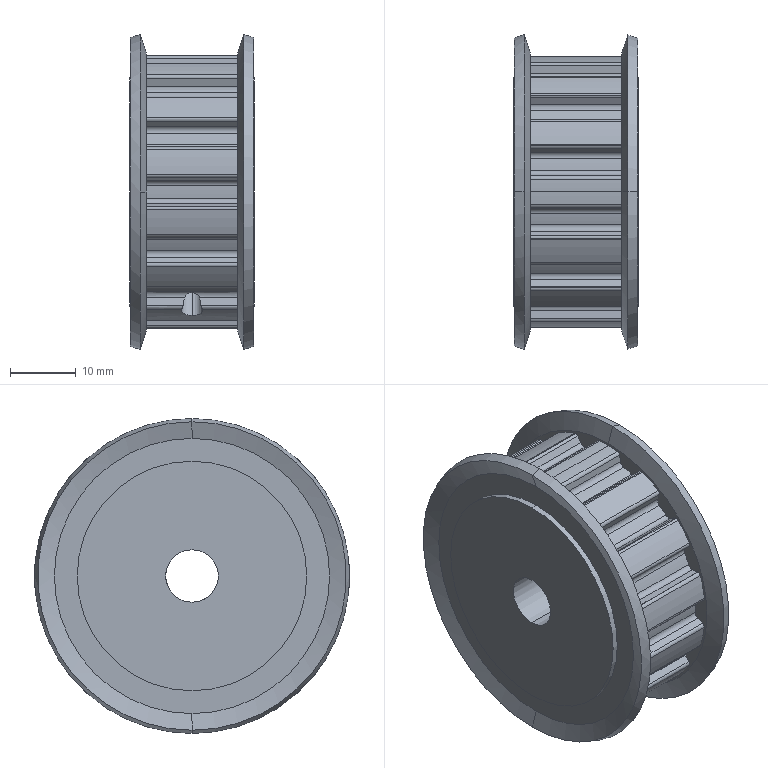Part | NX | features BREP 1 | 1 solid | 156 faces | box 19 x 48 x 48 mm | volume 23758 mm3 | cylinder 109 | plane 35 | cone 12 | commonest cylinder face diameters 1.06 x35 1.72 x34 37.42 x15 41.68 x15 3.242 x4 35 x4